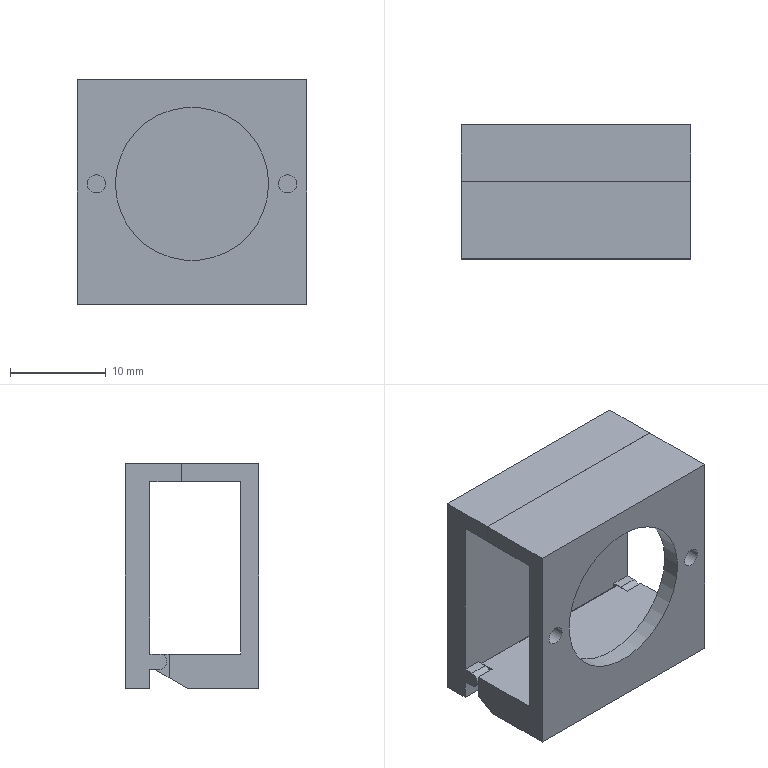Part | NX | 1 solid | 37 faces | box 24 x 14 x 23.5 mm | volume 3276 mm3 | plane 28 | cylinder 9 | commonest cylinder face diameters 1.9 x4 1.58 x2 16 x2 1.886 x1
STEP:
#1=CARTESIAN_POINT('',(11.99,14.,-12.59));
#2=VERTEX_POINT('',#1);
#3=CARTESIAN_POINT('',(-11.99,14.,-12.59));
#4=VERTEX_POINT('',#3);
#5=CARTESIAN_POINT('',(11.99,14.,-12.59));
#6=DIRECTION('',(-1.,0.,0.));
#7=VECTOR('',#6,1000.);
#8=LINE('',#5,#7);
#9=EDGE_CURVE('',#2,#4,#8,.T.);
#10=ORIENTED_EDGE('',*,*,#9,.T.);
#11=CARTESIAN_POINT('',(-11.99,14.,10.89));
#12=VERTEX_POINT('',#11);
#13=CARTESIAN_POINT('',(-11.99,14.,-12.59));
#14=DIRECTION('',(0.,0.,1.));
#15=VECTOR('',#14,1000.);
#16=LINE('',#13,#15);
#17=EDGE_CURVE('',#4,#12,#16,.T.);
#18=ORIENTED_EDGE('',*,*,#17,.T.);
#19=CARTESIAN_POINT('',(11.99,14.,10.89));
#20=VERTEX_POINT('',#19);
#21=CARTESIAN_POINT('',(-11.99,14.,10.89));
#22=DIRECTION('',(1.,0.,0.));
#23=VECTOR('',#22,1000.);
#24=LINE('',#21,#23);
#25=EDGE_CURVE('',#12,#20,#24,.T.);
#26=ORIENTED_EDGE('',*,*,#25,.T.);
#27=CARTESIAN_POINT('',(11.99,14.,10.89));
#28=DIRECTION('',(0.,0.,-1.));
#29=VECTOR('',#28,1000.);
#30=LINE('',#27,#29);
#31=EDGE_CURVE('',#20,#2,#30,.T.);
#32=ORIENTED_EDGE('',*,*,#31,.T.);
#33=EDGE_LOOP('',(#10,#18,#26,#32));
#34=FACE_BOUND('',#33,.T.);
#35=CARTESIAN_POINT('',(-12.,14.,-12.6));
#36=DIRECTION('',(0.,1.,0.));
#37=DIRECTION('',(1.,0.,0.));
#38=AXIS2_PLACEMENT_3D('',#35,#36,#37);
#39=PLANE('',#38);
#40=ADVANCED_FACE('',(#34),#39,.T.);
#41=ORIENTED_EDGE('',*,*,#9,.F.);
#42=CARTESIAN_POINT('',(11.99,11.4,-12.59));
#43=VERTEX_POINT('',#42);
#44=CARTESIAN_POINT('',(11.99,11.4,-12.59));
#45=DIRECTION('',(0.,1.,0.));
#46=VECTOR('',#45,1000.);
#47=LINE('',#44,#46);
#48=EDGE_CURVE('',#43,#2,#47,.T.);
#49=ORIENTED_EDGE('',*,*,#48,.F.);
#50=CARTESIAN_POINT('',(-11.99,11.4,-12.59));
#51=VERTEX_POINT('',#50);
#52=CARTESIAN_POINT('',(11.99,11.4,-12.59));
#53=DIRECTION('',(-1.,0.,0.));
#54=VECTOR('',#53,1000.);
#55=LINE('',#52,#54);
#56=EDGE_CURVE('',#43,#51,#55,.T.);
#57=ORIENTED_EDGE('',*,*,#56,.T.);
#58=CARTESIAN_POINT('',(-11.99,11.4,-12.59));
#59=DIRECTION('',(0.,1.,0.));
#60=VECTOR('',#59,1000.);
#61=LINE('',#58,#60);
#62=EDGE_CURVE('',#51,#4,#61,.T.);
#63=ORIENTED_EDGE('',*,*,#62,.T.);
#64=EDGE_LOOP('',(#41,#49,#57,#63));
#65=FACE_BOUND('',#64,.T.);
#66=CARTESIAN_POINT('',(-11.99,14.,-12.59));
#67=DIRECTION('',(0.,0.,1.));
#68=DIRECTION('',(1.,0.,0.));
#69=AXIS2_PLACEMENT_3D('',#66,#67,#68);
#70=PLANE('',#69);
#71=ADVANCED_FACE('',(#65),#70,.F.);
#72=ORIENTED_EDGE('',*,*,#17,.F.);
#73=ORIENTED_EDGE('',*,*,#62,.F.);
#74=CARTESIAN_POINT('',(-11.99,11.4,-10.59));
#75=VERTEX_POINT('',#74);
#76=CARTESIAN_POINT('',(-11.99,11.4,-12.59));
#77=DIRECTION('',(0.,0.,1.));
#78=VECTOR('',#77,1000.);
#79=LINE('',#76,#78);
#80=EDGE_CURVE('',#51,#75,#79,.T.);
#81=ORIENTED_EDGE('',*,*,#80,.T.);
#82=CARTESIAN_POINT('',(-11.99,10.4,-10.59));
#83=VERTEX_POINT('',#82);
#84=CARTESIAN_POINT('',(-11.99,10.4,-10.59));
#85=DIRECTION('',(0.,1.,0.));
#86=VECTOR('',#85,1000.);
#87=LINE('',#84,#86);
#88=EDGE_CURVE('',#83,#75,#87,.T.);
#89=ORIENTED_EDGE('',*,*,#88,.F.);
#90=CARTESIAN_POINT('',(-11.99,10.4,-9.01));
#91=VERTEX_POINT('',#90);
#92=CARTESIAN_POINT('',(-11.99,10.4,-9.8));
#93=DIRECTION('',(1.,0.,0.));
#94=DIRECTION('',(0.,0.,1.));
#95=AXIS2_PLACEMENT_3D('',#92,#93,#94);
#96=CIRCLE('',#95,0.79);
#97=EDGE_CURVE('',#91,#83,#96,.T.);
#98=ORIENTED_EDGE('',*,*,#97,.F.);
#99=CARTESIAN_POINT('',(-11.99,11.4,-9.01));
#100=VERTEX_POINT('',#99);
#101=CARTESIAN_POINT('',(-11.99,11.4,-9.01));
#102=DIRECTION('',(0.,-1.,0.));
#103=VECTOR('',#102,1000.);
#104=LINE('',#101,#103);
#105=EDGE_CURVE('',#100,#91,#104,.T.);
#106=ORIENTED_EDGE('',*,*,#105,.F.);
#107=CARTESIAN_POINT('',(-11.99,11.4,9.01));
#108=VERTEX_POINT('',#107);
#109=CARTESIAN_POINT('',(-11.99,11.4,-9.01));
#110=DIRECTION('',(0.,0.,1.));
#111=VECTOR('',#110,1000.);
#112=LINE('',#109,#111);
#113=EDGE_CURVE('',#100,#108,#112,.T.);
#114=ORIENTED_EDGE('',*,*,#113,.T.);
#115=CARTESIAN_POINT('',(-11.99,8.11,9.01));
#116=VERTEX_POINT('',#115);
#117=CARTESIAN_POINT('',(-11.99,8.11,9.01));
#118=DIRECTION('',(0.,1.,0.));
#119=VECTOR('',#118,1000.);
#120=LINE('',#117,#119);
#121=EDGE_CURVE('',#116,#108,#120,.T.);
#122=ORIENTED_EDGE('',*,*,#121,.F.);
#123=CARTESIAN_POINT('',(-11.99,8.11,10.89));
#124=VERTEX_POINT('',#123);
#125=CARTESIAN_POINT('',(-11.99,8.11,10.89));
#126=DIRECTION('',(0.,0.,-1.));
#127=VECTOR('',#126,1000.);
#128=LINE('',#125,#127);
#129=EDGE_CURVE('',#124,#116,#128,.T.);
#130=ORIENTED_EDGE('',*,*,#129,.F.);
#131=CARTESIAN_POINT('',(-11.99,8.11,10.89));
#132=DIRECTION('',(0.,1.,0.));
#133=VECTOR('',#132,1000.);
#134=LINE('',#131,#133);
#135=EDGE_CURVE('',#124,#12,#134,.T.);
#136=ORIENTED_EDGE('',*,*,#135,.T.);
#137=EDGE_LOOP('',(#72,#73,#81,#89,#98,#106,#114,#122,#130,#136));
#138=FACE_BOUND('',#137,.T.);
#139=CARTESIAN_POINT('',(-11.99,14.,10.89));
#140=DIRECTION('',(1.,0.,0.));
#141=DIRECTION('',(0.,1.,0.));
#142=AXIS2_PLACEMENT_3D('',#139,#140,#141);
#143=PLANE('',#142);
#144=ADVANCED_FACE('',(#138),#143,.F.);
#145=ORIENTED_EDGE('',*,*,#25,.F.);
#146=ORIENTED_EDGE('',*,*,#135,.F.);
#147=CARTESIAN_POINT('',(11.99,8.11,10.89));
#148=VERTEX_POINT('',#147);
#149=CARTESIAN_POINT('',(-11.99,8.11,10.89));
#150=DIRECTION('',(1.,0.,0.));
#151=VECTOR('',#150,1000.);
#152=LINE('',#149,#151);
#153=EDGE_CURVE('',#124,#148,#152,.T.);
#154=ORIENTED_EDGE('',*,*,#153,.T.);
#155=CARTESIAN_POINT('',(11.99,8.11,10.89));
#156=DIRECTION('',(0.,1.,0.));
#157=VECTOR('',#156,1000.);
#158=LINE('',#155,#157);
#159=EDGE_CURVE('',#148,#20,#158,.T.);
#160=ORIENTED_EDGE('',*,*,#159,.T.);
#161=EDGE_LOOP('',(#145,#146,#154,#160));
#162=FACE_BOUND('',#161,.T.);
#163=CARTESIAN_POINT('',(11.99,14.,10.89));
#164=DIRECTION('',(0.,0.,-1.));
#165=DIRECTION('',(0.,-1.,0.));
#166=AXIS2_PLACEMENT_3D('',#163,#164,#165);
#167=PLANE('',#166);
#168=ADVANCED_FACE('',(#162),#167,.F.);
#169=ORIENTED_EDGE('',*,*,#31,.F.);
#170=ORIENTED_EDGE('',*,*,#159,.F.);
#171=CARTESIAN_POINT('',(11.99,8.11,9.01));
#172=VERTEX_POINT('',#171);
#173=CARTESIAN_POINT('',(11.99,8.11,10.89));
#174=DIRECTION('',(0.,0.,-1.));
#175=VECTOR('',#174,1000.);
#176=LINE('',#173,#175);
#177=EDGE_CURVE('',#148,#172,#176,.T.);
#178=ORIENTED_EDGE('',*,*,#177,.T.);
#179=CARTESIAN_POINT('',(11.99,11.4,9.01));
#180=VERTEX_POINT('',#179);
#181=CARTESIAN_POINT('',(11.99,8.11,9.01));
#182=DIRECTION('',(0.,1.,0.));
#183=VECTOR('',#182,1000.);
#184=LINE('',#181,#183);
#185=EDGE_CURVE('',#172,#180,#184,.T.);
#186=ORIENTED_EDGE('',*,*,#185,.T.);
#187=CARTESIAN_POINT('',(11.99,11.4,-9.01));
#188=VERTEX_POINT('',#187);
#189=CARTESIAN_POINT('',(11.99,11.4,-9.01));
#190=DIRECTION('',(0.,0.,1.));
#191=VECTOR('',#190,1000.);
#192=LINE('',#189,#191);
#193=EDGE_CURVE('',#188,#180,#192,.T.);
#194=ORIENTED_EDGE('',*,*,#193,.F.);
#195=CARTESIAN_POINT('',(11.99,10.4,-9.01));
#196=VERTEX_POINT('',#195);
#197=CARTESIAN_POINT('',(11.99,11.4,-9.01));
#198=DIRECTION('',(0.,-1.,0.));
#199=VECTOR('',#198,1000.);
#200=LINE('',#197,#199);
#201=EDGE_CURVE('',#188,#196,#200,.T.);
#202=ORIENTED_EDGE('',*,*,#201,.T.);
#203=CARTESIAN_POINT('',(11.99,10.4,-10.59));
#204=VERTEX_POINT('',#203);
#205=CARTESIAN_POINT('',(11.99,10.4,-9.8));
#206=DIRECTION('',(-1.,0.,0.));
#207=DIRECTION('',(0.,0.,-1.));
#208=AXIS2_PLACEMENT_3D('',#205,#206,#207);
#209=CIRCLE('',#208,0.79);
#210=EDGE_CURVE('',#204,#196,#209,.T.);
#211=ORIENTED_EDGE('',*,*,#210,.F.);
#212=CARTESIAN_POINT('',(11.99,11.4,-10.59));
#213=VERTEX_POINT('',#212);
#214=CARTESIAN_POINT('',(11.99,10.4,-10.59));
#215=DIRECTION('',(0.,1.,0.));
#216=VECTOR('',#215,1000.);
#217=LINE('',#214,#216);
#218=EDGE_CURVE('',#204,#213,#217,.T.);
#219=ORIENTED_EDGE('',*,*,#218,.T.);
#220=CARTESIAN_POINT('',(11.99,11.4,-12.59));
#221=DIRECTION('',(0.,0.,1.));
#222=VECTOR('',#221,1000.);
#223=LINE('',#220,#222);
#224=EDGE_CURVE('',#43,#213,#223,.T.);
#225=ORIENTED_EDGE('',*,*,#224,.F.);
#226=ORIENTED_EDGE('',*,*,#48,.T.);
#227=EDGE_LOOP('',(#169,#170,#178,#186,#194,#202,#211,#219,#225,#226));
#228=FACE_BOUND('',#227,.T.);
#229=CARTESIAN_POINT('',(11.99,14.,-12.59));
#230=DIRECTION('',(-1.,0.,0.));
#231=DIRECTION('',(0.,0.,1.));
#232=AXIS2_PLACEMENT_3D('',#229,#230,#231);
#233=PLANE('',#232);
#234=ADVANCED_FACE('',(#228),#233,.F.);
#235=ORIENTED_EDGE('',*,*,#56,.F.);
#236=ORIENTED_EDGE('',*,*,#224,.T.);
#237=CARTESIAN_POINT('',(10.,11.4,-10.59));
#238=VERTEX_POINT('',#237);
#239=CARTESIAN_POINT('',(10.,11.4,-10.59));
#240=DIRECTION('',(1.,0.,0.));
#241=VECTOR('',#240,1000.);
#242=LINE('',#239,#241);
#243=EDGE_CURVE('',#238,#213,#242,.T.);
#244=ORIENTED_EDGE('',*,*,#243,.F.);
#245=CARTESIAN_POINT('',(10.,11.4,-9.01));
#246=VERTEX_POINT('',#245);
#247=CARTESIAN_POINT('',(10.,11.4,-9.01));
#248=DIRECTION('',(0.,0.,-1.));
#249=VECTOR('',#248,1000.);
#250=LINE('',#247,#249);
#251=EDGE_CURVE('',#246,#238,#250,.T.);
#252=ORIENTED_EDGE('',*,*,#251,.F.);
#253=CARTESIAN_POINT('',(10.,11.4,-9.01));
#254=DIRECTION('',(1.,0.,0.));
#255=VECTOR('',#254,1000.);
#256=LINE('',#253,#255);
#257=EDGE_CURVE('',#246,#188,#256,.T.);
#258=ORIENTED_EDGE('',*,*,#257,.T.);
#259=ORIENTED_EDGE('',*,*,#193,.T.);
#260=CARTESIAN_POINT('',(-11.99,11.4,9.01));
#261=DIRECTION('',(1.,0.,0.));
#262=VECTOR('',#261,1000.);
#263=LINE('',#260,#262);
#264=EDGE_CURVE('',#108,#180,#263,.T.);
#265=ORIENTED_EDGE('',*,*,#264,.F.);
#266=ORIENTED_EDGE('',*,*,#113,.F.);
#267=CARTESIAN_POINT('',(-10.,11.4,-9.01));
#268=VERTEX_POINT('',#267);
#269=CARTESIAN_POINT('',(-10.,11.4,-9.01));
#270=DIRECTION('',(-1.,0.,0.));
#271=VECTOR('',#270,1000.);
#272=LINE('',#269,#271);
#273=EDGE_CURVE('',#268,#100,#272,.T.);
#274=ORIENTED_EDGE('',*,*,#273,.F.);
#275=CARTESIAN_POINT('',(-10.,11.4,-10.59));
#276=VERTEX_POINT('',#275);
#277=CARTESIAN_POINT('',(-10.,11.4,-9.01));
#278=DIRECTION('',(0.,0.,-1.));
#279=VECTOR('',#278,1000.);
#280=LINE('',#277,#279);
#281=EDGE_CURVE('',#268,#276,#280,.T.);
#282=ORIENTED_EDGE('',*,*,#281,.T.);
#283=CARTESIAN_POINT('',(-10.,11.4,-10.59));
#284=DIRECTION('',(-1.,0.,0.));
#285=VECTOR('',#284,1000.);
#286=LINE('',#283,#285);
#287=EDGE_CURVE('',#276,#75,#286,.T.);
#288=ORIENTED_EDGE('',*,*,#287,.T.);
#289=ORIENTED_EDGE('',*,*,#80,.F.);
#290=EDGE_LOOP('',(#235,#236,#244,#252,#258,#259,#265,#266,#274,#282,#288,#289));
#291=FACE_BOUND('',#290,.T.);
#292=CARTESIAN_POINT('',(-12.,11.4,9.));
#293=DIRECTION('',(0.,-1.,0.));
#294=DIRECTION('',(0.,0.,-1.));
#295=AXIS2_PLACEMENT_3D('',#292,#293,#294);
#296=PLANE('',#295);
#297=ADVANCED_FACE('',(#291),#296,.T.);
#298=CARTESIAN_POINT('',(-10.,10.4,-10.59));
#299=VERTEX_POINT('',#298);
#300=CARTESIAN_POINT('',(-10.,10.4,-10.59));
#301=DIRECTION('',(-1.,0.,0.));
#302=VECTOR('',#301,1000.);
#303=LINE('',#300,#302);
#304=EDGE_CURVE('',#299,#83,#303,.T.);
#305=ORIENTED_EDGE('',*,*,#304,.T.);
#306=ORIENTED_EDGE('',*,*,#88,.T.);
#307=ORIENTED_EDGE('',*,*,#287,.F.);
#308=CARTESIAN_POINT('',(-10.,10.915,-10.59));
#309=VERTEX_POINT('',#308);
#310=CARTESIAN_POINT('',(-10.,10.915,-10.59));
#311=DIRECTION('',(0.,1.,0.));
#312=VECTOR('',#311,1000.);
#313=LINE('',#310,#312);
#314=EDGE_CURVE('',#309,#276,#313,.T.);
#315=ORIENTED_EDGE('',*,*,#314,.F.);
#316=CARTESIAN_POINT('',(-10.,10.4,-10.59));
#317=DIRECTION('',(0.,1.,0.));
#318=VECTOR('',#317,1000.);
#319=LINE('',#316,#318);
#320=EDGE_CURVE('',#299,#309,#319,.T.);
#321=ORIENTED_EDGE('',*,*,#320,.F.);
#322=EDGE_LOOP('',(#305,#306,#307,#315,#321));
#323=FACE_BOUND('',#322,.T.);
#324=CARTESIAN_POINT('',(-12.,11.4,-10.59));
#325=DIRECTION('',(0.,0.,-1.));
#326=DIRECTION('',(0.,-1.,0.));
#327=AXIS2_PLACEMENT_3D('',#324,#325,#326);
#328=PLANE('',#327);
#329=ADVANCED_FACE('',(#323),#328,.T.);
#330=ORIENTED_EDGE('',*,*,#97,.T.);
#331=ORIENTED_EDGE('',*,*,#304,.F.);
#332=CARTESIAN_POINT('',(-10.,10.4,-9.01));
#333=VERTEX_POINT('',#332);
#334=CARTESIAN_POINT('',(-10.,10.4,-9.8));
#335=DIRECTION('',(-1.,0.,0.));
#336=DIRECTION('',(0.,0.,-1.));
#337=AXIS2_PLACEMENT_3D('',#334,#335,#336);
#338=CIRCLE('',#337,0.79);
#339=EDGE_CURVE('',#299,#333,#338,.T.);
#340=ORIENTED_EDGE('',*,*,#339,.T.);
#341=CARTESIAN_POINT('',(-11.99,10.4,-9.01));
#342=DIRECTION('',(1.,0.,0.));
#343=VECTOR('',#342,1000.);
#344=LINE('',#341,#343);
#345=EDGE_CURVE('',#91,#333,#344,.T.);
#346=ORIENTED_EDGE('',*,*,#345,.F.);
#347=EDGE_LOOP('',(#330,#331,#340,#346));
#348=FACE_BOUND('',#347,.T.);
#349=CARTESIAN_POINT('',(-12.,10.4,-9.8));
#350=DIRECTION('',(1.,0.,0.));
#351=DIRECTION('',(0.,0.,-1.));
#352=AXIS2_PLACEMENT_3D('',#349,#350,#351);
#353=CYLINDRICAL_SURFACE('',#352,0.79);
#354=ADVANCED_FACE('',(#348),#353,.T.);
#355=ORIENTED_EDGE('',*,*,#105,.T.);
#356=ORIENTED_EDGE('',*,*,#345,.T.);
#357=CARTESIAN_POINT('',(-10.,10.915,-9.01));
#358=VERTEX_POINT('',#357);
#359=CARTESIAN_POINT('',(-10.,10.915,-9.01));
#360=DIRECTION('',(0.,-1.,0.));
#361=VECTOR('',#360,1000.);
#362=LINE('',#359,#361);
#363=EDGE_CURVE('',#358,#333,#362,.T.);
#364=ORIENTED_EDGE('',*,*,#363,.F.);
#365=CARTESIAN_POINT('',(-10.,10.915,-9.01));
#366=DIRECTION('',(0.,1.,0.));
#367=VECTOR('',#366,1000.);
#368=LINE('',#365,#367);
#369=EDGE_CURVE('',#358,#268,#368,.T.);
#370=ORIENTED_EDGE('',*,*,#369,.T.);
#371=ORIENTED_EDGE('',*,*,#273,.T.);
#372=EDGE_LOOP('',(#355,#356,#364,#370,#371));
#373=FACE_BOUND('',#372,.T.);
#374=CARTESIAN_POINT('',(-12.,10.4,-9.01));
#375=DIRECTION('',(0.,0.,1.));
#376=DIRECTION('',(1.,0.,0.));
#377=AXIS2_PLACEMENT_3D('',#374,#375,#376);
#378=PLANE('',#377);
#379=ADVANCED_FACE('',(#373),#378,.T.);
#380=ORIENTED_EDGE('',*,*,#281,.F.);
#381=ORIENTED_EDGE('',*,*,#369,.F.);
#382=CARTESIAN_POINT('',(-10.,10.4,-9.8));
#383=DIRECTION('',(1.,0.,0.));
#384=DIRECTION('',(0.,0.5458,-0.8379));
#385=AXIS2_PLACEMENT_3D('',#382,#383,#384);
#386=CIRCLE('',#385,0.9428);
#387=EDGE_CURVE('',#309,#358,#386,.T.);
#388=ORIENTED_EDGE('',*,*,#387,.F.);
#389=ORIENTED_EDGE('',*,*,#314,.T.);
#390=EDGE_LOOP('',(#380,#381,#388,#389));
#391=FACE_BOUND('',#390,.T.);
#392=CARTESIAN_POINT('',(-10.,0.,0.));
#393=DIRECTION('',(1.,0.,0.));
#394=DIRECTION('',(0.,1.,0.));
#395=AXIS2_PLACEMENT_3D('',#392,#393,#394);
#396=PLANE('',#395);
#397=ADVANCED_FACE('',(#391),#396,.T.);
#398=CARTESIAN_POINT('',(10.,10.899,-9.));
#399=VERTEX_POINT('',#398);
#400=CARTESIAN_POINT('',(-10.,10.899,-9.));
#401=VERTEX_POINT('',#400);
#402=CARTESIAN_POINT('',(10.,10.899,-9.));
#403=DIRECTION('',(-1.,0.,0.));
#404=VECTOR('',#403,1000.);
#405=LINE('',#402,#404);
#406=EDGE_CURVE('',#399,#401,#405,.T.);
#407=ORIENTED_EDGE('',*,*,#406,.F.);
#408=CARTESIAN_POINT('',(10.,10.915,-9.01));
#409=VERTEX_POINT('',#408);
#410=CARTESIAN_POINT('',(10.,10.4,-9.8));
#411=DIRECTION('',(-1.,0.,0.));
#412=DIRECTION('',(0.,0.5292,0.8485));
#413=AXIS2_PLACEMENT_3D('',#410,#411,#412);
#414=CIRCLE('',#413,0.9428);
#415=EDGE_CURVE('',#399,#409,#414,.T.);
#416=ORIENTED_EDGE('',*,*,#415,.T.);
#417=CARTESIAN_POINT('',(10.,10.915,-10.59));
#418=VERTEX_POINT('',#417);
#419=CARTESIAN_POINT('',(10.,10.4,-9.8));
#420=DIRECTION('',(-1.,0.,0.));
#421=DIRECTION('',(0.,0.5458,0.8379));
#422=AXIS2_PLACEMENT_3D('',#419,#420,#421);
#423=CIRCLE('',#422,0.9428);
#424=EDGE_CURVE('',#409,#418,#423,.T.);
#425=ORIENTED_EDGE('',*,*,#424,.T.);
#426=CARTESIAN_POINT('',(10.,10.899,-10.6));
#427=VERTEX_POINT('',#426);
#428=CARTESIAN_POINT('',(10.,10.899,-10.6));
#429=CARTESIAN_POINT('',(10.,10.904,-10.597));
#430=CARTESIAN_POINT('',(10.,10.909,-10.593));
#431=CARTESIAN_POINT('',(10.,10.915,-10.59));
#432=B_SPLINE_CURVE_WITH_KNOTS('',3,(#428,#429,#430,#431),.UNSPECIFIED.,.F.,.F.,(4,4),(0.,1.),.UNSPECIFIED.);
#433=EDGE_CURVE('',#418,#427,#432,.F.);
#434=ORIENTED_EDGE('',*,*,#433,.T.);
#435=CARTESIAN_POINT('',(-10.,10.899,-10.6));
#436=VERTEX_POINT('',#435);
#437=CARTESIAN_POINT('',(-10.,10.9,-10.6));
#438=CARTESIAN_POINT('',(-3.333,10.899,-10.6));
#439=CARTESIAN_POINT('',(3.333,10.899,-10.601));
#440=CARTESIAN_POINT('',(10.,10.899,-10.601));
#441=B_SPLINE_CURVE_WITH_KNOTS('',3,(#437,#438,#439,#440),.UNSPECIFIED.,.F.,.F.,(4,4),(0.,1.),.UNSPECIFIED.);
#442=EDGE_CURVE('',#436,#427,#441,.T.);
#443=ORIENTED_EDGE('',*,*,#442,.F.);
#444=CARTESIAN_POINT('',(-10.,10.4,-9.8));
#445=DIRECTION('',(1.,0.,0.));
#446=DIRECTION('',(0.,0.5297,-0.8482));
#447=AXIS2_PLACEMENT_3D('',#444,#445,#446);
#448=CIRCLE('',#447,0.9428);
#449=EDGE_CURVE('',#436,#309,#448,.T.);
#450=ORIENTED_EDGE('',*,*,#449,.T.);
#451=ORIENTED_EDGE('',*,*,#387,.T.);
#452=CARTESIAN_POINT('',(-10.,10.4,-9.8));
#453=DIRECTION('',(1.,0.,0.));
#454=DIRECTION('',(0.,0.5458,0.8379));
#455=AXIS2_PLACEMENT_3D('',#452,#453,#454);
#456=CIRCLE('',#455,0.9428);
#457=EDGE_CURVE('',#358,#401,#456,.T.);
#458=ORIENTED_EDGE('',*,*,#457,.T.);
#459=EDGE_LOOP('',(#407,#416,#425,#434,#443,#450,#451,#458));
#460=FACE_BOUND('',#459,.T.);
#461=CARTESIAN_POINT('',(10.,10.4,-9.8));
#462=DIRECTION('',(1.,0.,0.));
#463=DIRECTION('',(0.,0.,-1.));
#464=AXIS2_PLACEMENT_3D('',#461,#462,#463);
#465=CYLINDRICAL_SURFACE('',#464,0.9428);
#466=ADVANCED_FACE('',(#460),#465,.T.);
#467=ORIENTED_EDGE('',*,*,#406,.T.);
#468=CARTESIAN_POINT('',(-10.,9.4,-9.));
#469=VERTEX_POINT('',#468);
#470=CARTESIAN_POINT('',(-10.,10.899,-9.));
#471=DIRECTION('',(0.,-1.,0.));
#472=VECTOR('',#471,1000.);
#473=LINE('',#470,#472);
#474=EDGE_CURVE('',#401,#469,#473,.T.);
#475=ORIENTED_EDGE('',*,*,#474,.T.);
#476=CARTESIAN_POINT('',(-12.,9.4,-9.));
#477=VERTEX_POINT('',#476);
#478=CARTESIAN_POINT('',(-10.,9.4,-9.));
#479=DIRECTION('',(-1.,0.,0.));
#480=VECTOR('',#479,1000.);
#481=LINE('',#478,#480);
#482=EDGE_CURVE('',#469,#477,#481,.T.);
#483=ORIENTED_EDGE('',*,*,#482,.T.);
#484=CARTESIAN_POINT('',(-12.,1.9,-9.));
#485=VERTEX_POINT('',#484);
#486=CARTESIAN_POINT('',(-12.,1.9,-9.));
#487=DIRECTION('',(0.,1.,0.));
#488=VECTOR('',#487,1000.);
#489=LINE('',#486,#488);
#490=EDGE_CURVE('',#485,#477,#489,.T.);
#491=ORIENTED_EDGE('',*,*,#490,.F.);
#492=CARTESIAN_POINT('',(12.,1.9,-9.));
#493=VERTEX_POINT('',#492);
#494=CARTESIAN_POINT('',(12.,1.9,-9.));
#495=DIRECTION('',(-1.,0.,0.));
#496=VECTOR('',#495,1000.);
#497=LINE('',#494,#496);
#498=EDGE_CURVE('',#493,#485,#497,.T.);
#499=ORIENTED_EDGE('',*,*,#498,.F.);
#500=CARTESIAN_POINT('',(12.,9.4,-9.));
#501=VERTEX_POINT('',#500);
#502=CARTESIAN_POINT('',(12.,1.9,-9.));
#503=DIRECTION('',(0.,1.,0.));
#504=VECTOR('',#503,1000.);
#505=LINE('',#502,#504);
#506=EDGE_CURVE('',#493,#501,#505,.T.);
#507=ORIENTED_EDGE('',*,*,#506,.T.);
#508=CARTESIAN_POINT('',(10.,9.4,-9.));
#509=VERTEX_POINT('',#508);
#510=CARTESIAN_POINT('',(10.,9.4,-9.));
#511=DIRECTION('',(1.,0.,0.));
#512=VECTOR('',#511,1000.);
#513=LINE('',#510,#512);
#514=EDGE_CURVE('',#509,#501,#513,.T.);
#515=ORIENTED_EDGE('',*,*,#514,.F.);
#516=CARTESIAN_POINT('',(10.,10.899,-9.));
#517=DIRECTION('',(0.,-1.,0.));
#518=VECTOR('',#517,1000.);
#519=LINE('',#516,#518);
#520=EDGE_CURVE('',#399,#509,#519,.T.);
#521=ORIENTED_EDGE('',*,*,#520,.F.);
#522=EDGE_LOOP('',(#467,#475,#483,#491,#499,#507,#515,#521));
#523=FACE_BOUND('',#522,.T.);
#524=CARTESIAN_POINT('',(-12.,11.4,-9.));
#525=DIRECTION('',(0.,0.,1.));
#526=DIRECTION('',(1.,0.,0.));
#527=AXIS2_PLACEMENT_3D('',#524,#525,#526);
#528=PLANE('',#527);
#529=ADVANCED_FACE('',(#523),#528,.T.);
#530=CARTESIAN_POINT('',(10.,9.4,-11.466));
#531=VERTEX_POINT('',#530);
#532=CARTESIAN_POINT('',(10.,9.4,-11.466));
#533=CARTESIAN_POINT('',(10.,9.9,-11.178));
#534=CARTESIAN_POINT('',(10.,10.399,-10.889));
#535=CARTESIAN_POINT('',(10.,10.899,-10.6));
#536=B_SPLINE_CURVE_WITH_KNOTS('',3,(#532,#533,#534,#535),.UNSPECIFIED.,.F.,.F.,(4,4),(0.,1.),.UNSPECIFIED.);
#537=EDGE_CURVE('',#427,#531,#536,.F.);
#538=ORIENTED_EDGE('',*,*,#537,.F.);
#539=ORIENTED_EDGE('',*,*,#433,.F.);
#540=CARTESIAN_POINT('',(10.,10.4,-10.59));
#541=VERTEX_POINT('',#540);
#542=CARTESIAN_POINT('',(10.,10.4,-10.59));
#543=DIRECTION('',(0.,1.,0.));
#544=VECTOR('',#543,1000.);
#545=LINE('',#542,#544);
#546=EDGE_CURVE('',#541,#418,#545,.T.);
#547=ORIENTED_EDGE('',*,*,#546,.F.);
#548=CARTESIAN_POINT('',(10.,10.4,-9.01));
#549=VERTEX_POINT('',#548);
#550=CARTESIAN_POINT('',(10.,10.4,-9.8));
#551=DIRECTION('',(1.,0.,0.));
#552=DIRECTION('',(0.,0.,1.));
#553=AXIS2_PLACEMENT_3D('',#550,#551,#552);
#554=CIRCLE('',#553,0.79);
#555=EDGE_CURVE('',#549,#541,#554,.T.);
#556=ORIENTED_EDGE('',*,*,#555,.F.);
#557=CARTESIAN_POINT('',(10.,10.915,-9.01));
#558=DIRECTION('',(0.,-1.,0.));
#559=VECTOR('',#558,1000.);
#560=LINE('',#557,#559);
#561=EDGE_CURVE('',#409,#549,#560,.T.);
#562=ORIENTED_EDGE('',*,*,#561,.F.);
#563=ORIENTED_EDGE('',*,*,#415,.F.);
#564=ORIENTED_EDGE('',*,*,#520,.T.);
#565=CARTESIAN_POINT('',(10.,9.4,-11.466));
#566=DIRECTION('',(0.,0.,1.));
#567=VECTOR('',#566,1000.);
#568=LINE('',#565,#567);
#569=EDGE_CURVE('',#531,#509,#568,.T.);
#570=ORIENTED_EDGE('',*,*,#569,.F.);
#571=EDGE_LOOP('',(#538,#539,#547,#556,#562,#563,#564,#570));
#572=FACE_BOUND('',#571,.T.);
#573=CARTESIAN_POINT('',(10.,0.,0.));
#574=DIRECTION('',(1.,0.,0.));
#575=DIRECTION('',(0.,1.,0.));
#576=AXIS2_PLACEMENT_3D('',#573,#574,#575);
#577=PLANE('',#576);
#578=ADVANCED_FACE('',(#572),#577,.T.);
#579=ORIENTED_EDGE('',*,*,#442,.T.);
#580=ORIENTED_EDGE('',*,*,#537,.T.);
#581=CARTESIAN_POINT('',(12.,9.4,-11.466));
#582=VERTEX_POINT('',#581);
#583=CARTESIAN_POINT('',(10.,9.4,-11.466));
#584=DIRECTION('',(1.,0.,0.));
#585=VECTOR('',#584,1000.);
#586=LINE('',#583,#585);
#587=EDGE_CURVE('',#531,#582,#586,.T.);
#588=ORIENTED_EDGE('',*,*,#587,.T.);
#589=CARTESIAN_POINT('',(12.,7.436,-12.6));
#590=VERTEX_POINT('',#589);
#591=CARTESIAN_POINT('',(12.,9.4,-11.466));
#592=DIRECTION('',(0.,-0.866,-0.5));
#593=VECTOR('',#592,1000.);
#594=LINE('',#591,#593);
#595=EDGE_CURVE('',#582,#590,#594,.T.);
#596=ORIENTED_EDGE('',*,*,#595,.T.);
#597=CARTESIAN_POINT('',(-12.,7.436,-12.6));
#598=VERTEX_POINT('',#597);
#599=CARTESIAN_POINT('',(12.,7.436,-12.6));
#600=DIRECTION('',(-1.,0.,0.));
#601=VECTOR('',#600,1000.);
#602=LINE('',#599,#601);
#603=EDGE_CURVE('',#590,#598,#602,.T.);
#604=ORIENTED_EDGE('',*,*,#603,.T.);
#605=CARTESIAN_POINT('',(-12.,9.4,-11.466));
#606=VERTEX_POINT('',#605);
#607=CARTESIAN_POINT('',(-12.,7.436,-12.6));
#608=DIRECTION('',(0.,0.866,0.5));
#609=VECTOR('',#608,1000.);
#610=LINE('',#607,#609);
#611=EDGE_CURVE('',#598,#606,#610,.T.);
#612=ORIENTED_EDGE('',*,*,#611,.T.);
#613=CARTESIAN_POINT('',(-10.,9.4,-11.466));
#614=VERTEX_POINT('',#613);
#615=CARTESIAN_POINT('',(-10.,9.4,-11.466));
#616=DIRECTION('',(-1.,0.,0.));
#617=VECTOR('',#616,1000.);
#618=LINE('',#615,#617);
#619=EDGE_CURVE('',#614,#606,#618,.T.);
#620=ORIENTED_EDGE('',*,*,#619,.F.);
#621=CARTESIAN_POINT('',(-10.,9.4,-11.466));
#622=CARTESIAN_POINT('',(-10.,9.9,-11.177));
#623=CARTESIAN_POINT('',(-10.,10.4,-10.889));
#624=CARTESIAN_POINT('',(-10.,10.9,-10.6));
#625=B_SPLINE_CURVE_WITH_KNOTS('',3,(#621,#622,#623,#624),.UNSPECIFIED.,.F.,.F.,(4,4),(0.,1.),.UNSPECIFIED.);
#626=EDGE_CURVE('',#614,#436,#625,.T.);
#627=ORIENTED_EDGE('',*,*,#626,.T.);
#628=EDGE_LOOP('',(#579,#580,#588,#596,#604,#612,#620,#627));
#629=FACE_BOUND('',#628,.T.);
#630=CARTESIAN_POINT('',(12.,10.9,-10.6));
#631=DIRECTION('',(0.,-0.5,0.866));
#632=DIRECTION('',(-1.,0.,0.));
#633=AXIS2_PLACEMENT_3D('',#630,#631,#632);
#634=PLANE('',#633);
#635=ADVANCED_FACE('',(#629),#634,.F.);
#636=ORIENTED_EDGE('',*,*,#626,.F.);
#637=CARTESIAN_POINT('',(-10.,9.4,-11.466));
#638=DIRECTION('',(0.,0.,1.));
#639=VECTOR('',#638,1000.);
#640=LINE('',#637,#639);
#641=EDGE_CURVE('',#614,#469,#640,.T.);
#642=ORIENTED_EDGE('',*,*,#641,.T.);
#643=ORIENTED_EDGE('',*,*,#474,.F.);
#644=ORIENTED_EDGE('',*,*,#457,.F.);
#645=ORIENTED_EDGE('',*,*,#363,.T.);
#646=ORIENTED_EDGE('',*,*,#339,.F.);
#647=ORIENTED_EDGE('',*,*,#320,.T.);
#648=ORIENTED_EDGE('',*,*,#449,.F.);
#649=EDGE_LOOP('',(#636,#642,#643,#644,#645,#646,#647,#648));
#650=FACE_BOUND('',#649,.T.);
#651=CARTESIAN_POINT('',(-10.,0.,0.));
#652=DIRECTION('',(1.,0.,0.));
#653=DIRECTION('',(0.,1.,0.));
#654=AXIS2_PLACEMENT_3D('',#651,#652,#653);
#655=PLANE('',#654);
#656=ADVANCED_FACE('',(#650),#655,.F.);
#657=CARTESIAN_POINT('',(-12.,9.4,-11.466));
#658=DIRECTION('',(0.,0.,1.));
#659=VECTOR('',#658,1000.);
#660=LINE('',#657,#659);
#661=EDGE_CURVE('',#606,#477,#660,.T.);
#662=ORIENTED_EDGE('',*,*,#661,.T.);
#663=ORIENTED_EDGE('',*,*,#482,.F.);
#664=ORIENTED_EDGE('',*,*,#641,.F.);
#665=ORIENTED_EDGE('',*,*,#619,.T.);
#666=EDGE_LOOP('',(#662,#663,#664,#665));
#667=FACE_BOUND('',#666,.T.);
#668=CARTESIAN_POINT('',(-12.,9.4,-9.));
#669=DIRECTION('',(0.,1.,0.));
#670=DIRECTION('',(1.,0.,0.));
#671=AXIS2_PLACEMENT_3D('',#668,#669,#670);
#672=PLANE('',#671);
#673=ADVANCED_FACE('',(#667),#672,.T.);
#674=ORIENTED_EDGE('',*,*,#661,.F.);
#675=ORIENTED_EDGE('',*,*,#611,.F.);
#676=CARTESIAN_POINT('',(-12.,0.,-12.6));
#677=VERTEX_POINT('',#676);
#678=CARTESIAN_POINT('',(-12.,7.436,-12.6));
#679=DIRECTION('',(0.,-1.,0.));
#680=VECTOR('',#679,1000.);
#681=LINE('',#678,#680);
#682=EDGE_CURVE('',#598,#677,#681,.T.);
#683=ORIENTED_EDGE('',*,*,#682,.T.);
#684=CARTESIAN_POINT('',(-12.,0.,10.9));
#685=VERTEX_POINT('',#684);
#686=CARTESIAN_POINT('',(-12.,0.,-12.6));
#687=DIRECTION('',(0.,0.,1.));
#688=VECTOR('',#687,1000.);
#689=LINE('',#686,#688);
#690=EDGE_CURVE('',#677,#685,#689,.T.);
#691=ORIENTED_EDGE('',*,*,#690,.T.);
#692=CARTESIAN_POINT('',(-12.,8.1,10.9));
#693=VERTEX_POINT('',#692);
#694=CARTESIAN_POINT('',(-12.,0.,10.9));
#695=DIRECTION('',(0.,1.,0.));
#696=VECTOR('',#695,1000.);
#697=LINE('',#694,#696);
#698=EDGE_CURVE('',#685,#693,#697,.T.);
#699=ORIENTED_EDGE('',*,*,#698,.T.);
#700=CARTESIAN_POINT('',(-12.,8.1,9.));
#701=VERTEX_POINT('',#700);
#702=CARTESIAN_POINT('',(-12.,8.1,10.9));
#703=DIRECTION('',(0.,0.,-1.));
#704=VECTOR('',#703,1000.);
#705=LINE('',#702,#704);
#706=EDGE_CURVE('',#693,#701,#705,.T.);
#707=ORIENTED_EDGE('',*,*,#706,.T.);
#708=CARTESIAN_POINT('',(-12.,1.9,9.));
#709=VERTEX_POINT('',#708);
#710=CARTESIAN_POINT('',(-12.,8.1,9.));
#711=DIRECTION('',(0.,-1.,0.));
#712=VECTOR('',#711,1000.);
#713=LINE('',#710,#712);
#714=EDGE_CURVE('',#701,#709,#713,.T.);
#715=ORIENTED_EDGE('',*,*,#714,.T.);
#716=CARTESIAN_POINT('',(-12.,1.9,9.));
#717=DIRECTION('',(0.,0.,-1.));
#718=VECTOR('',#717,1000.);
#719=LINE('',#716,#718);
#720=EDGE_CURVE('',#709,#485,#719,.T.);
#721=ORIENTED_EDGE('',*,*,#720,.T.);
#722=ORIENTED_EDGE('',*,*,#490,.T.);
#723=EDGE_LOOP('',(#674,#675,#683,#691,#699,#707,#715,#721,#722));
#724=FACE_BOUND('',#723,.T.);
#725=CARTESIAN_POINT('',(-12.,0.,0.));
#726=DIRECTION('',(1.,0.,0.));
#727=DIRECTION('',(0.,1.,0.));
#728=AXIS2_PLACEMENT_3D('',#725,#726,#727);
#729=PLANE('',#728);
#730=ADVANCED_FACE('',(#724),#729,.F.);
#731=ORIENTED_EDGE('',*,*,#720,.F.);
#732=CARTESIAN_POINT('',(12.,1.9,9.));
#733=VERTEX_POINT('',#732);
#734=CARTESIAN_POINT('',(12.,1.9,9.));
#735=DIRECTION('',(-1.,0.,0.));
#736=VECTOR('',#735,1000.);
#737=LINE('',#734,#736);
#738=EDGE_CURVE('',#733,#709,#737,.T.);
#739=ORIENTED_EDGE('',*,*,#738,.F.);
#740=CARTESIAN_POINT('',(12.,1.9,9.));
#741=DIRECTION('',(0.,0.,-1.));
#742=VECTOR('',#741,1000.);
#743=LINE('',#740,#742);
#744=EDGE_CURVE('',#733,#493,#743,.T.);
#745=ORIENTED_EDGE('',*,*,#744,.T.);
#746=ORIENTED_EDGE('',*,*,#498,.T.);
#747=EDGE_LOOP('',(#731,#739,#745,#746));
#748=FACE_BOUND('',#747,.T.);
#749=CARTESIAN_POINT('',(8.,1.9,0.));
#750=VERTEX_POINT('',#749);
#751=CARTESIAN_POINT('',(-8.,1.9,0.));
#752=VERTEX_POINT('',#751);
#753=CARTESIAN_POINT('',(0.,1.9,0.));
#754=DIRECTION('',(0.,1.,0.));
#755=DIRECTION('',(-1.,0.,0.));
#756=AXIS2_PLACEMENT_3D('',#753,#754,#755);
#757=CIRCLE('',#756,8.);
#758=EDGE_CURVE('',#750,#752,#757,.T.);
#759=ORIENTED_EDGE('',*,*,#758,.F.);
#760=CARTESIAN_POINT('',(0.,1.9,0.));
#761=DIRECTION('',(0.,1.,0.));
#762=DIRECTION('',(-1.,0.,0.));
#763=AXIS2_PLACEMENT_3D('',#760,#761,#762);
#764=CIRCLE('',#763,8.);
#765=EDGE_CURVE('',#752,#750,#764,.T.);
#766=ORIENTED_EDGE('',*,*,#765,.F.);
#767=EDGE_LOOP('',(#759,#766));
#768=FACE_BOUND('',#767,.T.);
#769=CARTESIAN_POINT('',(10.95,1.9,0.));
#770=VERTEX_POINT('',#769);
#771=CARTESIAN_POINT('',(9.05,1.9,0.));
#772=VERTEX_POINT('',#771);
#773=CARTESIAN_POINT('',(10.,1.9,0.));
#774=DIRECTION('',(0.,1.,0.));
#775=DIRECTION('',(-1.,0.,0.));
#776=AXIS2_PLACEMENT_3D('',#773,#774,#775);
#777=CIRCLE('',#776,0.95);
#778=EDGE_CURVE('',#770,#772,#777,.T.);
#779=ORIENTED_EDGE('',*,*,#778,.F.);
#780=CARTESIAN_POINT('',(10.,1.9,0.));
#781=DIRECTION('',(0.,1.,0.));
#782=DIRECTION('',(-1.,0.,0.));
#783=AXIS2_PLACEMENT_3D('',#780,#781,#782);
#784=CIRCLE('',#783,0.95);
#785=EDGE_CURVE('',#772,#770,#784,.T.);
#786=ORIENTED_EDGE('',*,*,#785,.F.);
#787=EDGE_LOOP('',(#779,#786));
#788=FACE_BOUND('',#787,.T.);
#789=CARTESIAN_POINT('',(-10.95,1.9,0.));
#790=VERTEX_POINT('',#789);
#791=CARTESIAN_POINT('',(-9.05,1.9,0.));
#792=VERTEX_POINT('',#791);
#793=CARTESIAN_POINT('',(-10.,1.9,0.));
#794=DIRECTION('',(0.,1.,0.));
#795=DIRECTION('',(-1.,0.,0.));
#796=AXIS2_PLACEMENT_3D('',#793,#794,#795);
#797=CIRCLE('',#796,0.95);
#798=EDGE_CURVE('',#790,#792,#797,.T.);
#799=ORIENTED_EDGE('',*,*,#798,.F.);
#800=CARTESIAN_POINT('',(-10.,1.9,0.));
#801=DIRECTION('',(0.,1.,0.));
#802=DIRECTION('',(-1.,0.,0.));
#803=AXIS2_PLACEMENT_3D('',#800,#801,#802);
#804=CIRCLE('',#803,0.95);
#805=EDGE_CURVE('',#792,#790,#804,.T.);
#806=ORIENTED_EDGE('',*,*,#805,.F.);
#807=EDGE_LOOP('',(#799,#806));
#808=FACE_BOUND('',#807,.T.);
#809=CARTESIAN_POINT('',(-12.,1.9,-9.));
#810=DIRECTION('',(0.,1.,0.));
#811=DIRECTION('',(1.,0.,0.));
#812=AXIS2_PLACEMENT_3D('',#809,#810,#811);
#813=PLANE('',#812);
#814=ADVANCED_FACE('',(#748,#768,#788,#808),#813,.T.);
#815=CARTESIAN_POINT('',(12.,9.4,-11.466));
#816=DIRECTION('',(0.,0.,1.));
#817=VECTOR('',#816,1000.);
#818=LINE('',#815,#817);
#819=EDGE_CURVE('',#582,#501,#818,.T.);
#820=ORIENTED_EDGE('',*,*,#819,.T.);
#821=ORIENTED_EDGE('',*,*,#506,.F.);
#822=ORIENTED_EDGE('',*,*,#744,.F.);
#823=CARTESIAN_POINT('',(12.,8.1,9.));
#824=VERTEX_POINT('',#823);
#825=CARTESIAN_POINT('',(12.,8.1,9.));
#826=DIRECTION('',(0.,-1.,0.));
#827=VECTOR('',#826,1000.);
#828=LINE('',#825,#827);
#829=EDGE_CURVE('',#824,#733,#828,.T.);
#830=ORIENTED_EDGE('',*,*,#829,.F.);
#831=CARTESIAN_POINT('',(12.,8.1,10.9));
#832=VERTEX_POINT('',#831);
#833=CARTESIAN_POINT('',(12.,8.1,10.9));
#834=DIRECTION('',(0.,0.,-1.));
#835=VECTOR('',#834,1000.);
#836=LINE('',#833,#835);
#837=EDGE_CURVE('',#832,#824,#836,.T.);
#838=ORIENTED_EDGE('',*,*,#837,.F.);
#839=CARTESIAN_POINT('',(12.,0.,10.9));
#840=VERTEX_POINT('',#839);
#841=CARTESIAN_POINT('',(12.,0.,10.9));
#842=DIRECTION('',(0.,1.,0.));
#843=VECTOR('',#842,1000.);
#844=LINE('',#841,#843);
#845=EDGE_CURVE('',#840,#832,#844,.T.);
#846=ORIENTED_EDGE('',*,*,#845,.F.);
#847=CARTESIAN_POINT('',(12.,0.,-12.6));
#848=VERTEX_POINT('',#847);
#849=CARTESIAN_POINT('',(12.,0.,-12.6));
#850=DIRECTION('',(0.,0.,1.));
#851=VECTOR('',#850,1000.);
#852=LINE('',#849,#851);
#853=EDGE_CURVE('',#848,#840,#852,.T.);
#854=ORIENTED_EDGE('',*,*,#853,.F.);
#855=CARTESIAN_POINT('',(12.,7.436,-12.6));
#856=DIRECTION('',(0.,-1.,0.));
#857=VECTOR('',#856,1000.);
#858=LINE('',#855,#857);
#859=EDGE_CURVE('',#590,#848,#858,.T.);
#860=ORIENTED_EDGE('',*,*,#859,.F.);
#861=ORIENTED_EDGE('',*,*,#595,.F.);
#862=EDGE_LOOP('',(#820,#821,#822,#830,#838,#846,#854,#860,#861));
#863=FACE_BOUND('',#862,.T.);
#864=CARTESIAN_POINT('',(12.,0.,0.));
#865=DIRECTION('',(1.,0.,0.));
#866=DIRECTION('',(0.,1.,0.));
#867=AXIS2_PLACEMENT_3D('',#864,#865,#866);
#868=PLANE('',#867);
#869=ADVANCED_FACE('',(#863),#868,.T.);
#870=ORIENTED_EDGE('',*,*,#819,.F.);
#871=ORIENTED_EDGE('',*,*,#587,.F.);
#872=ORIENTED_EDGE('',*,*,#569,.T.);
#873=ORIENTED_EDGE('',*,*,#514,.T.);
#874=EDGE_LOOP('',(#870,#871,#872,#873));
#875=FACE_BOUND('',#874,.T.);
#876=CARTESIAN_POINT('',(12.,9.4,-9.));
#877=DIRECTION('',(0.,-1.,0.));
#878=DIRECTION('',(0.,0.,-1.));
#879=AXIS2_PLACEMENT_3D('',#876,#877,#878);
#880=PLANE('',#879);
#881=ADVANCED_FACE('',(#875),#880,.F.);
#882=ORIENTED_EDGE('',*,*,#682,.F.);
#883=ORIENTED_EDGE('',*,*,#603,.F.);
#884=ORIENTED_EDGE('',*,*,#859,.T.);
#885=CARTESIAN_POINT('',(12.,0.,-12.6));
#886=DIRECTION('',(-1.,0.,0.));
#887=VECTOR('',#886,1000.);
#888=LINE('',#885,#887);
#889=EDGE_CURVE('',#848,#677,#888,.T.);
#890=ORIENTED_EDGE('',*,*,#889,.T.);
#891=EDGE_LOOP('',(#882,#883,#884,#890));
#892=FACE_BOUND('',#891,.T.);
#893=CARTESIAN_POINT('',(-12.,0.,-12.6));
#894=DIRECTION('',(0.,0.,-1.));
#895=DIRECTION('',(0.,-1.,0.));
#896=AXIS2_PLACEMENT_3D('',#893,#894,#895);
#897=PLANE('',#896);
#898=ADVANCED_FACE('',(#892),#897,.T.);
#899=ORIENTED_EDGE('',*,*,#690,.F.);
#900=ORIENTED_EDGE('',*,*,#889,.F.);
#901=ORIENTED_EDGE('',*,*,#853,.T.);
#902=CARTESIAN_POINT('',(12.,0.,10.9));
#903=DIRECTION('',(-1.,0.,0.));
#904=VECTOR('',#903,1000.);
#905=LINE('',#902,#904);
#906=EDGE_CURVE('',#840,#685,#905,.T.);
#907=ORIENTED_EDGE('',*,*,#906,.T.);
#908=EDGE_LOOP('',(#899,#900,#901,#907));
#909=FACE_BOUND('',#908,.T.);
#910=CARTESIAN_POINT('',(-8.,0.,0.));
#911=VERTEX_POINT('',#910);
#912=CARTESIAN_POINT('',(8.,0.,0.));
#913=VERTEX_POINT('',#912);
#914=CARTESIAN_POINT('',(0.,0.,0.));
#915=DIRECTION('',(0.,-1.,0.));
#916=DIRECTION('',(1.,0.,0.));
#917=AXIS2_PLACEMENT_3D('',#914,#915,#916);
#918=CIRCLE('',#917,8.);
#919=EDGE_CURVE('',#911,#913,#918,.T.);
#920=ORIENTED_EDGE('',*,*,#919,.F.);
#921=CARTESIAN_POINT('',(0.,0.,0.));
#922=DIRECTION('',(0.,-1.,0.));
#923=DIRECTION('',(1.,0.,0.));
#924=AXIS2_PLACEMENT_3D('',#921,#922,#923);
#925=CIRCLE('',#924,8.);
#926=EDGE_CURVE('',#913,#911,#925,.T.);
#927=ORIENTED_EDGE('',*,*,#926,.F.);
#928=EDGE_LOOP('',(#920,#927));
#929=FACE_BOUND('',#928,.T.);
#930=CARTESIAN_POINT('',(9.05,0.,0.));
#931=VERTEX_POINT('',#930);
#932=CARTESIAN_POINT('',(10.95,0.,0.));
#933=VERTEX_POINT('',#932);
#934=CARTESIAN_POINT('',(10.,0.,0.));
#935=DIRECTION('',(0.,-1.,0.));
#936=DIRECTION('',(1.,0.,0.));
#937=AXIS2_PLACEMENT_3D('',#934,#935,#936);
#938=CIRCLE('',#937,0.95);
#939=EDGE_CURVE('',#931,#933,#938,.T.);
#940=ORIENTED_EDGE('',*,*,#939,.F.);
#941=CARTESIAN_POINT('',(10.,0.,0.));
#942=DIRECTION('',(0.,-1.,0.));
#943=DIRECTION('',(1.,0.,0.));
#944=AXIS2_PLACEMENT_3D('',#941,#942,#943);
#945=CIRCLE('',#944,0.95);
#946=EDGE_CURVE('',#933,#931,#945,.T.);
#947=ORIENTED_EDGE('',*,*,#946,.F.);
#948=EDGE_LOOP('',(#940,#947));
#949=FACE_BOUND('',#948,.T.);
#950=CARTESIAN_POINT('',(-9.05,0.,0.));
#951=VERTEX_POINT('',#950);
#952=CARTESIAN_POINT('',(-10.95,0.,0.));
#953=VERTEX_POINT('',#952);
#954=CARTESIAN_POINT('',(-10.,0.,0.));
#955=DIRECTION('',(0.,-1.,0.));
#956=DIRECTION('',(1.,0.,0.));
#957=AXIS2_PLACEMENT_3D('',#954,#955,#956);
#958=CIRCLE('',#957,0.95);
#959=EDGE_CURVE('',#951,#953,#958,.T.);
#960=ORIENTED_EDGE('',*,*,#959,.F.);
#961=CARTESIAN_POINT('',(-10.,0.,0.));
#962=DIRECTION('',(0.,-1.,0.));
#963=DIRECTION('',(1.,0.,0.));
#964=AXIS2_PLACEMENT_3D('',#961,#962,#963);
#965=CIRCLE('',#964,0.95);
#966=EDGE_CURVE('',#953,#951,#965,.T.);
#967=ORIENTED_EDGE('',*,*,#966,.F.);
#968=EDGE_LOOP('',(#960,#967));
#969=FACE_BOUND('',#968,.T.);
#970=CARTESIAN_POINT('',(-12.,0.,10.9));
#971=DIRECTION('',(0.,-1.,0.));
#972=DIRECTION('',(0.,0.,-1.));
#973=AXIS2_PLACEMENT_3D('',#970,#971,#972);
#974=PLANE('',#973);
#975=ADVANCED_FACE('',(#909,#929,#949,#969),#974,.T.);
#976=ORIENTED_EDGE('',*,*,#698,.F.);
#977=ORIENTED_EDGE('',*,*,#906,.F.);
#978=ORIENTED_EDGE('',*,*,#845,.T.);
#979=CARTESIAN_POINT('',(12.,8.1,10.9));
#980=DIRECTION('',(-1.,0.,0.));
#981=VECTOR('',#980,1000.);
#982=LINE('',#979,#981);
#983=EDGE_CURVE('',#832,#693,#982,.T.);
#984=ORIENTED_EDGE('',*,*,#983,.T.);
#985=EDGE_LOOP('',(#976,#977,#978,#984));
#986=FACE_BOUND('',#985,.T.);
#987=CARTESIAN_POINT('',(-12.,14.,10.9));
#988=DIRECTION('',(0.,0.,1.));
#989=DIRECTION('',(1.,0.,0.));
#990=AXIS2_PLACEMENT_3D('',#987,#988,#989);
#991=PLANE('',#990);
#992=ADVANCED_FACE('',(#986),#991,.T.);
#993=ORIENTED_EDGE('',*,*,#706,.F.);
#994=ORIENTED_EDGE('',*,*,#983,.F.);
#995=ORIENTED_EDGE('',*,*,#837,.T.);
#996=CARTESIAN_POINT('',(12.,8.1,9.));
#997=DIRECTION('',(-1.,0.,0.));
#998=VECTOR('',#997,1000.);
#999=LINE('',#996,#998);
#1000=EDGE_CURVE('',#824,#701,#999,.T.);
#1001=ORIENTED_EDGE('',*,*,#1000,.T.);
#1002=EDGE_LOOP('',(#993,#994,#995,#1001));
#1003=FACE_BOUND('',#1002,.T.);
#1004=CARTESIAN_POINT('',(12.,8.1,10.9));
#1005=DIRECTION('',(0.,-1.,0.));
#1006=DIRECTION('',(0.,0.,-1.));
#1007=AXIS2_PLACEMENT_3D('',#1004,#1005,#1006);
#1008=PLANE('',#1007);
#1009=ADVANCED_FACE('',(#1003),#1008,.F.);
#1010=ORIENTED_EDGE('',*,*,#714,.F.);
#1011=ORIENTED_EDGE('',*,*,#1000,.F.);
#1012=ORIENTED_EDGE('',*,*,#829,.T.);
#1013=ORIENTED_EDGE('',*,*,#738,.T.);
#1014=EDGE_LOOP('',(#1010,#1011,#1012,#1013));
#1015=FACE_BOUND('',#1014,.T.);
#1016=CARTESIAN_POINT('',(-12.,1.9,9.));
#1017=DIRECTION('',(0.,0.,-1.));
#1018=DIRECTION('',(0.,-1.,0.));
#1019=AXIS2_PLACEMENT_3D('',#1016,#1017,#1018);
#1020=PLANE('',#1019);
#1021=ADVANCED_FACE('',(#1015),#1020,.T.);
#1022=ORIENTED_EDGE('',*,*,#919,.T.);
#1023=CARTESIAN_POINT('',(8.,1.9,0.));
#1024=DIRECTION('',(0.,1.,0.));
#1025=VECTOR('',#1024,1000.);
#1026=LINE('',#1023,#1025);
#1027=EDGE_CURVE('',#913,#750,#1026,.T.);
#1028=ORIENTED_EDGE('',*,*,#1027,.T.);
#1029=ORIENTED_EDGE('',*,*,#758,.T.);
#1030=CARTESIAN_POINT('',(-8.,1.9,0.));
#1031=DIRECTION('',(0.,1.,0.));
#1032=VECTOR('',#1031,1000.);
#1033=LINE('',#1030,#1032);
#1034=EDGE_CURVE('',#911,#752,#1033,.T.);
#1035=ORIENTED_EDGE('',*,*,#1034,.F.);
#1036=EDGE_LOOP('',(#1022,#1028,#1029,#1035));
#1037=FACE_BOUND('',#1036,.T.);
#1038=CARTESIAN_POINT('',(0.,1.9,0.));
#1039=DIRECTION('',(0.,1.,0.));
#1040=DIRECTION('',(1.,0.,0.));
#1041=AXIS2_PLACEMENT_3D('',#1038,#1039,#1040);
#1042=CYLINDRICAL_SURFACE('',#1041,8.);
#1043=ADVANCED_FACE('',(#1037),#1042,.F.);
#1044=ORIENTED_EDGE('',*,*,#251,.T.);
#1045=CARTESIAN_POINT('',(10.,10.915,-10.59));
#1046=DIRECTION('',(0.,1.,0.));
#1047=VECTOR('',#1046,1000.);
#1048=LINE('',#1045,#1047);
#1049=EDGE_CURVE('',#418,#238,#1048,.T.);
#1050=ORIENTED_EDGE('',*,*,#1049,.F.);
#1051=ORIENTED_EDGE('',*,*,#424,.F.);
#1052=CARTESIAN_POINT('',(10.,10.915,-9.01));
#1053=DIRECTION('',(0.,1.,0.));
#1054=VECTOR('',#1053,1000.);
#1055=LINE('',#1052,#1054);
#1056=EDGE_CURVE('',#409,#246,#1055,.T.);
#1057=ORIENTED_EDGE('',*,*,#1056,.T.);
#1058=EDGE_LOOP('',(#1044,#1050,#1051,#1057));
#1059=FACE_BOUND('',#1058,.T.);
#1060=CARTESIAN_POINT('',(10.,0.,0.));
#1061=DIRECTION('',(1.,0.,0.));
#1062=DIRECTION('',(0.,1.,0.));
#1063=AXIS2_PLACEMENT_3D('',#1060,#1061,#1062);
#1064=PLANE('',#1063);
#1065=ADVANCED_FACE('',(#1059),#1064,.F.);
#1066=ORIENTED_EDGE('',*,*,#939,.T.);
#1067=CARTESIAN_POINT('',(10.95,1.9,0.));
#1068=DIRECTION('',(0.,1.,0.));
#1069=VECTOR('',#1068,1000.);
#1070=LINE('',#1067,#1069);
#1071=EDGE_CURVE('',#933,#770,#1070,.T.);
#1072=ORIENTED_EDGE('',*,*,#1071,.T.);
#1073=ORIENTED_EDGE('',*,*,#778,.T.);
#1074=CARTESIAN_POINT('',(9.05,1.9,0.));
#1075=DIRECTION('',(0.,1.,0.));
#1076=VECTOR('',#1075,1000.);
#1077=LINE('',#1074,#1076);
#1078=EDGE_CURVE('',#931,#772,#1077,.T.);
#1079=ORIENTED_EDGE('',*,*,#1078,.F.);
#1080=EDGE_LOOP('',(#1066,#1072,#1073,#1079));
#1081=FACE_BOUND('',#1080,.T.);
#1082=CARTESIAN_POINT('',(10.,1.9,0.));
#1083=DIRECTION('',(0.,1.,0.));
#1084=DIRECTION('',(1.,0.,0.));
#1085=AXIS2_PLACEMENT_3D('',#1082,#1083,#1084);
#1086=CYLINDRICAL_SURFACE('',#1085,0.95);
#1087=ADVANCED_FACE('',(#1081),#1086,.F.);
#1088=ORIENTED_EDGE('',*,*,#177,.F.);
#1089=ORIENTED_EDGE('',*,*,#153,.F.);
#1090=ORIENTED_EDGE('',*,*,#129,.T.);
#1091=CARTESIAN_POINT('',(-11.99,8.11,9.01));
#1092=DIRECTION('',(1.,0.,0.));
#1093=VECTOR('',#1092,1000.);
#1094=LINE('',#1091,#1093);
#1095=EDGE_CURVE('',#116,#172,#1094,.T.);
#1096=ORIENTED_EDGE('',*,*,#1095,.T.);
#1097=EDGE_LOOP('',(#1088,#1089,#1090,#1096));
#1098=FACE_BOUND('',#1097,.T.);
#1099=CARTESIAN_POINT('',(12.,8.11,9.01));
#1100=DIRECTION('',(0.,1.,0.));
#1101=DIRECTION('',(1.,0.,0.));
#1102=AXIS2_PLACEMENT_3D('',#1099,#1100,#1101);
#1103=PLANE('',#1102);
#1104=ADVANCED_FACE('',(#1098),#1103,.F.);
#1105=ORIENTED_EDGE('',*,*,#959,.T.);
#1106=CARTESIAN_POINT('',(-10.95,1.9,0.));
#1107=DIRECTION('',(0.,1.,0.));
#1108=VECTOR('',#1107,1000.);
#1109=LINE('',#1106,#1108);
#1110=EDGE_CURVE('',#953,#790,#1109,.T.);
#1111=ORIENTED_EDGE('',*,*,#1110,.T.);
#1112=ORIENTED_EDGE('',*,*,#798,.T.);
#1113=CARTESIAN_POINT('',(-9.05,1.9,0.));
#1114=DIRECTION('',(0.,1.,0.));
#1115=VECTOR('',#1114,1000.);
#1116=LINE('',#1113,#1115);
#1117=EDGE_CURVE('',#951,#792,#1116,.T.);
#1118=ORIENTED_EDGE('',*,*,#1117,.F.);
#1119=EDGE_LOOP('',(#1105,#1111,#1112,#1118));
#1120=FACE_BOUND('',#1119,.T.);
#1121=CARTESIAN_POINT('',(-10.,1.9,0.));
#1122=DIRECTION('',(0.,1.,0.));
#1123=DIRECTION('',(1.,0.,0.));
#1124=AXIS2_PLACEMENT_3D('',#1121,#1122,#1123);
#1125=CYLINDRICAL_SURFACE('',#1124,0.95);
#1126=ADVANCED_FACE('',(#1120),#1125,.F.);
#1127=ORIENTED_EDGE('',*,*,#185,.F.);
#1128=ORIENTED_EDGE('',*,*,#1095,.F.);
#1129=ORIENTED_EDGE('',*,*,#121,.T.);
#1130=ORIENTED_EDGE('',*,*,#264,.T.);
#1131=EDGE_LOOP('',(#1127,#1128,#1129,#1130));
#1132=FACE_BOUND('',#1131,.T.);
#1133=CARTESIAN_POINT('',(12.,11.4,9.01));
#1134=DIRECTION('',(0.,0.,1.));
#1135=DIRECTION('',(1.,0.,0.));
#1136=AXIS2_PLACEMENT_3D('',#1133,#1134,#1135);
#1137=PLANE('',#1136);
#1138=ADVANCED_FACE('',(#1132),#1137,.F.);
#1139=ORIENTED_EDGE('',*,*,#201,.F.);
#1140=ORIENTED_EDGE('',*,*,#257,.F.);
#1141=ORIENTED_EDGE('',*,*,#1056,.F.);
#1142=ORIENTED_EDGE('',*,*,#561,.T.);
#1143=CARTESIAN_POINT('',(10.,10.4,-9.01));
#1144=DIRECTION('',(1.,0.,0.));
#1145=VECTOR('',#1144,1000.);
#1146=LINE('',#1143,#1145);
#1147=EDGE_CURVE('',#549,#196,#1146,.T.);
#1148=ORIENTED_EDGE('',*,*,#1147,.T.);
#1149=EDGE_LOOP('',(#1139,#1140,#1141,#1142,#1148));
#1150=FACE_BOUND('',#1149,.T.);
#1151=CARTESIAN_POINT('',(12.,10.4,-9.01));
#1152=DIRECTION('',(0.,0.,-1.));
#1153=DIRECTION('',(0.,-1.,0.));
#1154=AXIS2_PLACEMENT_3D('',#1151,#1152,#1153);
#1155=PLANE('',#1154);
#1156=ADVANCED_FACE('',(#1150),#1155,.F.);
#1157=ORIENTED_EDGE('',*,*,#210,.T.);
#1158=ORIENTED_EDGE('',*,*,#1147,.F.);
#1159=ORIENTED_EDGE('',*,*,#555,.T.);
#1160=CARTESIAN_POINT('',(11.99,10.4,-10.59));
#1161=DIRECTION('',(-1.,0.,0.));
#1162=VECTOR('',#1161,1000.);
#1163=LINE('',#1160,#1162);
#1164=EDGE_CURVE('',#204,#541,#1163,.T.);
#1165=ORIENTED_EDGE('',*,*,#1164,.F.);
#1166=EDGE_LOOP('',(#1157,#1158,#1159,#1165));
#1167=FACE_BOUND('',#1166,.T.);
#1168=CARTESIAN_POINT('',(12.,10.4,-9.8));
#1169=DIRECTION('',(1.,0.,0.));
#1170=DIRECTION('',(0.,0.,-1.));
#1171=AXIS2_PLACEMENT_3D('',#1168,#1169,#1170);
#1172=CYLINDRICAL_SURFACE('',#1171,0.79);
#1173=ADVANCED_FACE('',(#1167),#1172,.T.);
#1174=ORIENTED_EDGE('',*,*,#1164,.T.);
#1175=ORIENTED_EDGE('',*,*,#546,.T.);
#1176=ORIENTED_EDGE('',*,*,#1049,.T.);
#1177=ORIENTED_EDGE('',*,*,#243,.T.);
#1178=ORIENTED_EDGE('',*,*,#218,.F.);
#1179=EDGE_LOOP('',(#1174,#1175,#1176,#1177,#1178));
#1180=FACE_BOUND('',#1179,.T.);
#1181=CARTESIAN_POINT('',(12.,11.4,-10.59));
#1182=DIRECTION('',(0.,0.,1.));
#1183=DIRECTION('',(1.,0.,0.));
#1184=AXIS2_PLACEMENT_3D('',#1181,#1182,#1183);
#1185=PLANE('',#1184);
#1186=ADVANCED_FACE('',(#1180),#1185,.F.);
#1187=ORIENTED_EDGE('',*,*,#1027,.F.);
#1188=ORIENTED_EDGE('',*,*,#926,.T.);
#1189=ORIENTED_EDGE('',*,*,#1034,.T.);
#1190=ORIENTED_EDGE('',*,*,#765,.T.);
#1191=EDGE_LOOP('',(#1187,#1188,#1189,#1190));
#1192=FACE_BOUND('',#1191,.T.);
#1193=CARTESIAN_POINT('',(0.,1.9,0.));
#1194=DIRECTION('',(0.,1.,0.));
#1195=DIRECTION('',(1.,0.,0.));
#1196=AXIS2_PLACEMENT_3D('',#1193,#1194,#1195);
#1197=CYLINDRICAL_SURFACE('',#1196,8.);
#1198=ADVANCED_FACE('',(#1192),#1197,.F.);
#1199=ORIENTED_EDGE('',*,*,#1117,.T.);
#1200=ORIENTED_EDGE('',*,*,#805,.T.);
#1201=ORIENTED_EDGE('',*,*,#1110,.F.);
#1202=ORIENTED_EDGE('',*,*,#966,.T.);
#1203=EDGE_LOOP('',(#1199,#1200,#1201,#1202));
#1204=FACE_BOUND('',#1203,.T.);
#1205=CARTESIAN_POINT('',(-10.,1.9,0.));
#1206=DIRECTION('',(0.,1.,0.));
#1207=DIRECTION('',(1.,0.,0.));
#1208=AXIS2_PLACEMENT_3D('',#1205,#1206,#1207);
#1209=CYLINDRICAL_SURFACE('',#1208,0.95);
#1210=ADVANCED_FACE('',(#1204),#1209,.F.);
#1211=ORIENTED_EDGE('',*,*,#1071,.F.);
#1212=ORIENTED_EDGE('',*,*,#946,.T.);
#1213=ORIENTED_EDGE('',*,*,#1078,.T.);
#1214=ORIENTED_EDGE('',*,*,#785,.T.);
#1215=EDGE_LOOP('',(#1211,#1212,#1213,#1214));
#1216=FACE_BOUND('',#1215,.T.);
#1217=CARTESIAN_POINT('',(10.,1.9,0.));
#1218=DIRECTION('',(0.,1.,0.));
#1219=DIRECTION('',(1.,0.,0.));
#1220=AXIS2_PLACEMENT_3D('',#1217,#1218,#1219);
#1221=CYLINDRICAL_SURFACE('',#1220,0.95);
#1222=ADVANCED_FACE('',(#1216),#1221,.F.);
#1223=CLOSED_SHELL('',(#40,#71,#144,#168,#234,#297,#329,#354,#379,#397,#466,#529,#578,#635,#656,#673,#730,#814,#869,#881,#898,#975,#992,#1009,#1021,#1043,#1065,#1087,#1104,#1126,#1138,#1156,#1173,#1186,#1198,#1210,#1222));
#1224=MANIFOLD_SOLID_BREP('',#1223);
#1225=(LENGTH_UNIT()NAMED_UNIT(*)SI_UNIT(.MILLI.,.METRE.));
#1226=UNCERTAINTY_MEASURE_WITH_UNIT(LENGTH_MEASURE(0.0508),#1225,'','');
#1227=(NAMED_UNIT(*)PLANE_ANGLE_UNIT()SI_UNIT($,.RADIAN.));
#1228=(NAMED_UNIT(*)SI_UNIT($,.STERADIAN.)SOLID_ANGLE_UNIT());
#1229=(GEOMETRIC_REPRESENTATION_CONTEXT(3)GLOBAL_UNCERTAINTY_ASSIGNED_CONTEXT((#1226))GLOBAL_UNIT_ASSIGNED_CONTEXT((#1225,#1227,#1228))REPRESENTATION_CONTEXT('',''));
#1230=ADVANCED_BREP_SHAPE_REPRESENTATION('',(#1224),#1229);